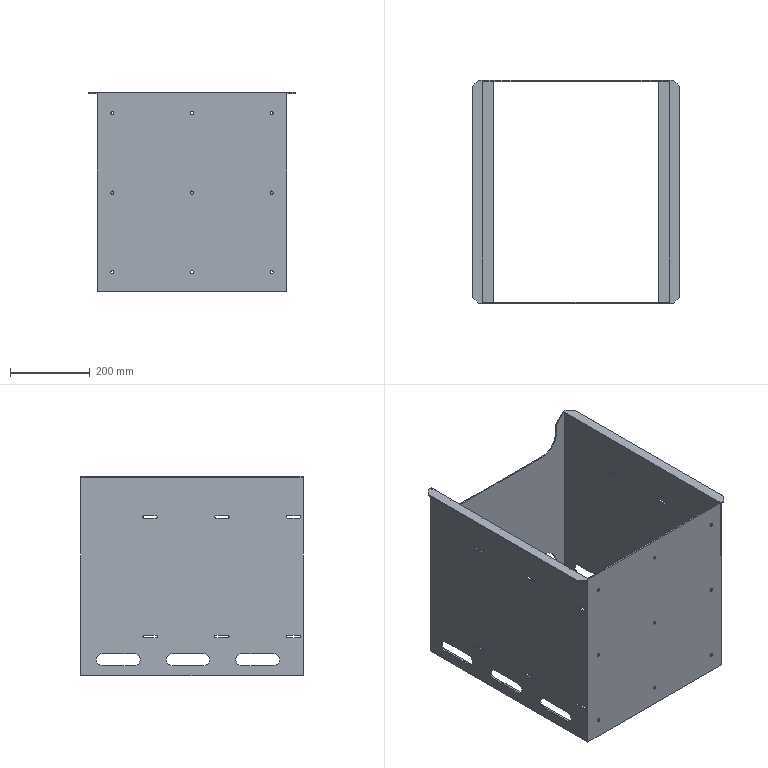Part | STEP file | Electrical cabinet box | 1 solid | 122 faces | box 520 x 560 x 500 mm | volume 2941429 mm3 | plane 64 | cylinder 58 | commonest cylinder face diameters 6.2 x24 8.2 x18 30 x12 100 x4